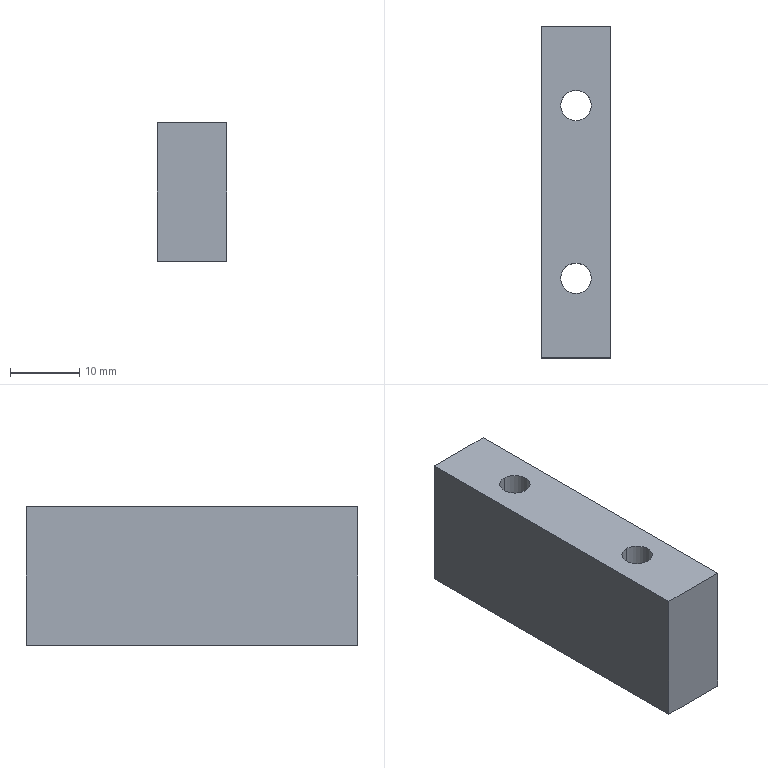Part | SolidWorks | features Extrusion 1, HoleWzd 1 | 1 solid | 16 faces | box 10 x 48 x 20 mm | volume 8641 mm3 | cylinder 8 | plane 8 | commonest cylinder face diameters 4.4 x4 8 x4
STEP:
#1=CARTESIAN_POINT('',(5.,-16.5,-5.));
#2=VERTEX_POINT('',#1);
#3=CARTESIAN_POINT('',(5.,-8.5,-5.));
#4=VERTEX_POINT('',#3);
#5=CARTESIAN_POINT('',(5.,-12.5,-5.));
#6=DIRECTION('',(0.,0.,-1.));
#7=DIRECTION('',(0.,1.,0.));
#8=AXIS2_PLACEMENT_3D('',#5,#6,#7);
#9=CIRCLE('',#8,4.);
#10=EDGE_CURVE('',#2,#4,#9,.T.);
#11=ORIENTED_EDGE('',*,*,#10,.F.);
#12=CARTESIAN_POINT('',(5.,-16.5,-10.));
#13=VERTEX_POINT('',#12);
#14=CARTESIAN_POINT('',(5.,-16.5,-10.));
#15=DIRECTION('',(0.,0.,-1.));
#16=VECTOR('',#15,1000.);
#17=LINE('',#14,#16);
#18=EDGE_CURVE('',#2,#13,#17,.T.);
#19=ORIENTED_EDGE('',*,*,#18,.T.);
#20=CARTESIAN_POINT('',(5.,-8.5,-10.));
#21=VERTEX_POINT('',#20);
#22=CARTESIAN_POINT('',(5.,-12.5,-10.));
#23=DIRECTION('',(0.,0.,-1.));
#24=DIRECTION('',(0.,1.,0.));
#25=AXIS2_PLACEMENT_3D('',#22,#23,#24);
#26=CIRCLE('',#25,4.);
#27=EDGE_CURVE('',#13,#21,#26,.T.);
#28=ORIENTED_EDGE('',*,*,#27,.T.);
#29=CARTESIAN_POINT('',(5.,-8.5,-10.));
#30=DIRECTION('',(0.,0.,-1.));
#31=VECTOR('',#30,1000.);
#32=LINE('',#29,#31);
#33=EDGE_CURVE('',#4,#21,#32,.T.);
#34=ORIENTED_EDGE('',*,*,#33,.F.);
#35=EDGE_LOOP('',(#11,#19,#28,#34));
#36=FACE_OUTER_BOUND('',#35,.T.);
#37=CARTESIAN_POINT('',(5.,-12.5,-10.));
#38=DIRECTION('',(0.,0.,-1.));
#39=DIRECTION('',(0.,1.,0.));
#40=AXIS2_PLACEMENT_3D('',#37,#38,#39);
#41=CYLINDRICAL_SURFACE('',#40,4.);
#42=ADVANCED_FACE('',(#36),#41,.F.);
#43=CARTESIAN_POINT('',(5.,-14.7,10.));
#44=VERTEX_POINT('',#43);
#45=CARTESIAN_POINT('',(5.,-10.3,10.));
#46=VERTEX_POINT('',#45);
#47=CARTESIAN_POINT('',(5.,-12.5,10.));
#48=DIRECTION('',(0.,0.,-1.));
#49=DIRECTION('',(0.,1.,0.));
#50=AXIS2_PLACEMENT_3D('',#47,#48,#49);
#51=CIRCLE('',#50,2.2);
#52=EDGE_CURVE('',#44,#46,#51,.T.);
#53=ORIENTED_EDGE('',*,*,#52,.F.);
#54=CARTESIAN_POINT('',(5.,-14.7,-5.));
#55=VERTEX_POINT('',#54);
#56=CARTESIAN_POINT('',(5.,-14.7,-10.));
#57=DIRECTION('',(0.,0.,-1.));
#58=VECTOR('',#57,1000.);
#59=LINE('',#56,#58);
#60=EDGE_CURVE('',#44,#55,#59,.T.);
#61=ORIENTED_EDGE('',*,*,#60,.T.);
#62=CARTESIAN_POINT('',(5.,-10.3,-5.));
#63=VERTEX_POINT('',#62);
#64=CARTESIAN_POINT('',(5.,-12.5,-5.));
#65=DIRECTION('',(0.,0.,-1.));
#66=DIRECTION('',(0.,1.,0.));
#67=AXIS2_PLACEMENT_3D('',#64,#65,#66);
#68=CIRCLE('',#67,2.2);
#69=EDGE_CURVE('',#55,#63,#68,.T.);
#70=ORIENTED_EDGE('',*,*,#69,.T.);
#71=CARTESIAN_POINT('',(5.,-10.3,-10.));
#72=DIRECTION('',(0.,0.,-1.));
#73=VECTOR('',#72,1000.);
#74=LINE('',#71,#73);
#75=EDGE_CURVE('',#46,#63,#74,.T.);
#76=ORIENTED_EDGE('',*,*,#75,.F.);
#77=EDGE_LOOP('',(#53,#61,#70,#76));
#78=FACE_OUTER_BOUND('',#77,.T.);
#79=CARTESIAN_POINT('',(5.,-12.5,-10.));
#80=DIRECTION('',(0.,0.,-1.));
#81=DIRECTION('',(0.,1.,0.));
#82=AXIS2_PLACEMENT_3D('',#79,#80,#81);
#83=CYLINDRICAL_SURFACE('',#82,2.2);
#84=ADVANCED_FACE('',(#78),#83,.F.);
#85=CARTESIAN_POINT('',(5.,8.5,-5.));
#86=VERTEX_POINT('',#85);
#87=CARTESIAN_POINT('',(5.,16.5,-5.));
#88=VERTEX_POINT('',#87);
#89=CARTESIAN_POINT('',(5.,12.5,-5.));
#90=DIRECTION('',(0.,0.,-1.));
#91=DIRECTION('',(0.,1.,0.));
#92=AXIS2_PLACEMENT_3D('',#89,#90,#91);
#93=CIRCLE('',#92,4.);
#94=EDGE_CURVE('',#86,#88,#93,.T.);
#95=ORIENTED_EDGE('',*,*,#94,.F.);
#96=CARTESIAN_POINT('',(5.,8.5,-10.));
#97=VERTEX_POINT('',#96);
#98=CARTESIAN_POINT('',(5.,8.5,-10.));
#99=DIRECTION('',(0.,0.,-1.));
#100=VECTOR('',#99,1000.);
#101=LINE('',#98,#100);
#102=EDGE_CURVE('',#86,#97,#101,.T.);
#103=ORIENTED_EDGE('',*,*,#102,.T.);
#104=CARTESIAN_POINT('',(5.,16.5,-10.));
#105=VERTEX_POINT('',#104);
#106=CARTESIAN_POINT('',(5.,12.5,-10.));
#107=DIRECTION('',(0.,0.,-1.));
#108=DIRECTION('',(0.,1.,0.));
#109=AXIS2_PLACEMENT_3D('',#106,#107,#108);
#110=CIRCLE('',#109,4.);
#111=EDGE_CURVE('',#97,#105,#110,.T.);
#112=ORIENTED_EDGE('',*,*,#111,.T.);
#113=CARTESIAN_POINT('',(5.,16.5,-10.));
#114=DIRECTION('',(0.,0.,-1.));
#115=VECTOR('',#114,1000.);
#116=LINE('',#113,#115);
#117=EDGE_CURVE('',#88,#105,#116,.T.);
#118=ORIENTED_EDGE('',*,*,#117,.F.);
#119=EDGE_LOOP('',(#95,#103,#112,#118));
#120=FACE_OUTER_BOUND('',#119,.T.);
#121=CARTESIAN_POINT('',(5.,12.5,-10.));
#122=DIRECTION('',(0.,0.,-1.));
#123=DIRECTION('',(0.,1.,0.));
#124=AXIS2_PLACEMENT_3D('',#121,#122,#123);
#125=CYLINDRICAL_SURFACE('',#124,4.);
#126=ADVANCED_FACE('',(#120),#125,.F.);
#127=CARTESIAN_POINT('',(5.,10.3,10.));
#128=VERTEX_POINT('',#127);
#129=CARTESIAN_POINT('',(5.,14.7,10.));
#130=VERTEX_POINT('',#129);
#131=CARTESIAN_POINT('',(5.,12.5,10.));
#132=DIRECTION('',(0.,0.,-1.));
#133=DIRECTION('',(0.,1.,0.));
#134=AXIS2_PLACEMENT_3D('',#131,#132,#133);
#135=CIRCLE('',#134,2.2);
#136=EDGE_CURVE('',#128,#130,#135,.T.);
#137=ORIENTED_EDGE('',*,*,#136,.F.);
#138=CARTESIAN_POINT('',(5.,10.3,-5.));
#139=VERTEX_POINT('',#138);
#140=CARTESIAN_POINT('',(5.,10.3,-10.));
#141=DIRECTION('',(0.,0.,-1.));
#142=VECTOR('',#141,1000.);
#143=LINE('',#140,#142);
#144=EDGE_CURVE('',#128,#139,#143,.T.);
#145=ORIENTED_EDGE('',*,*,#144,.T.);
#146=CARTESIAN_POINT('',(5.,14.7,-5.));
#147=VERTEX_POINT('',#146);
#148=CARTESIAN_POINT('',(5.,12.5,-5.));
#149=DIRECTION('',(0.,0.,-1.));
#150=DIRECTION('',(0.,1.,0.));
#151=AXIS2_PLACEMENT_3D('',#148,#149,#150);
#152=CIRCLE('',#151,2.2);
#153=EDGE_CURVE('',#139,#147,#152,.T.);
#154=ORIENTED_EDGE('',*,*,#153,.T.);
#155=CARTESIAN_POINT('',(5.,14.7,-10.));
#156=DIRECTION('',(0.,0.,-1.));
#157=VECTOR('',#156,1000.);
#158=LINE('',#155,#157);
#159=EDGE_CURVE('',#130,#147,#158,.T.);
#160=ORIENTED_EDGE('',*,*,#159,.F.);
#161=EDGE_LOOP('',(#137,#145,#154,#160));
#162=FACE_OUTER_BOUND('',#161,.T.);
#163=CARTESIAN_POINT('',(5.,12.5,-10.));
#164=DIRECTION('',(0.,0.,-1.));
#165=DIRECTION('',(0.,1.,0.));
#166=AXIS2_PLACEMENT_3D('',#163,#164,#165);
#167=CYLINDRICAL_SURFACE('',#166,2.2);
#168=ADVANCED_FACE('',(#162),#167,.F.);
#169=CARTESIAN_POINT('',(5.,-12.5,-10.));
#170=DIRECTION('',(0.,0.,-1.));
#171=DIRECTION('',(0.,1.,0.));
#172=AXIS2_PLACEMENT_3D('',#169,#170,#171);
#173=CIRCLE('',#172,4.);
#174=EDGE_CURVE('',#21,#13,#173,.T.);
#175=ORIENTED_EDGE('',*,*,#174,.F.);
#176=ORIENTED_EDGE('',*,*,#27,.F.);
#177=EDGE_LOOP('',(#175,#176));
#178=FACE_BOUND('',#177,.T.);
#179=CARTESIAN_POINT('',(5.,12.5,-10.));
#180=DIRECTION('',(0.,0.,-1.));
#181=DIRECTION('',(0.,1.,0.));
#182=AXIS2_PLACEMENT_3D('',#179,#180,#181);
#183=CIRCLE('',#182,4.);
#184=EDGE_CURVE('',#105,#97,#183,.T.);
#185=ORIENTED_EDGE('',*,*,#184,.F.);
#186=ORIENTED_EDGE('',*,*,#111,.F.);
#187=EDGE_LOOP('',(#185,#186));
#188=FACE_BOUND('',#187,.T.);
#189=CARTESIAN_POINT('',(0.,-24.,-10.));
#190=VERTEX_POINT('',#189);
#191=CARTESIAN_POINT('',(0.,24.,-10.));
#192=VERTEX_POINT('',#191);
#193=CARTESIAN_POINT('',(0.,24.,-10.));
#194=DIRECTION('',(0.,1.,0.));
#195=VECTOR('',#194,1000.);
#196=LINE('',#193,#195);
#197=EDGE_CURVE('',#190,#192,#196,.T.);
#198=ORIENTED_EDGE('',*,*,#197,.T.);
#199=CARTESIAN_POINT('',(10.,24.,-10.));
#200=VERTEX_POINT('',#199);
#201=CARTESIAN_POINT('',(10.,24.,-10.));
#202=DIRECTION('',(-1.,0.,0.));
#203=VECTOR('',#202,1000.);
#204=LINE('',#201,#203);
#205=EDGE_CURVE('',#200,#192,#204,.T.);
#206=ORIENTED_EDGE('',*,*,#205,.F.);
#207=CARTESIAN_POINT('',(10.,-24.,-10.));
#208=VERTEX_POINT('',#207);
#209=CARTESIAN_POINT('',(10.,24.,-10.));
#210=DIRECTION('',(0.,1.,0.));
#211=VECTOR('',#210,1000.);
#212=LINE('',#209,#211);
#213=EDGE_CURVE('',#208,#200,#212,.T.);
#214=ORIENTED_EDGE('',*,*,#213,.F.);
#215=CARTESIAN_POINT('',(10.,-24.,-10.));
#216=DIRECTION('',(-1.,0.,0.));
#217=VECTOR('',#216,1000.);
#218=LINE('',#215,#217);
#219=EDGE_CURVE('',#208,#190,#218,.T.);
#220=ORIENTED_EDGE('',*,*,#219,.T.);
#221=EDGE_LOOP('',(#198,#206,#214,#220));
#222=FACE_OUTER_BOUND('',#221,.T.);
#223=CARTESIAN_POINT('',(10.,24.,-10.));
#224=DIRECTION('',(0.,0.,1.));
#225=DIRECTION('',(0.,-1.,0.));
#226=AXIS2_PLACEMENT_3D('',#223,#224,#225);
#227=PLANE('',#226);
#228=ADVANCED_FACE('',(#178,#188,#222),#227,.F.);
#229=CARTESIAN_POINT('',(0.,24.,10.));
#230=VERTEX_POINT('',#229);
#231=CARTESIAN_POINT('',(0.,24.,10.));
#232=DIRECTION('',(0.,0.,1.));
#233=VECTOR('',#232,1000.);
#234=LINE('',#231,#233);
#235=EDGE_CURVE('',#192,#230,#234,.T.);
#236=ORIENTED_EDGE('',*,*,#235,.T.);
#237=CARTESIAN_POINT('',(10.,24.,10.));
#238=VERTEX_POINT('',#237);
#239=CARTESIAN_POINT('',(10.,24.,10.));
#240=DIRECTION('',(-1.,0.,0.));
#241=VECTOR('',#240,1000.);
#242=LINE('',#239,#241);
#243=EDGE_CURVE('',#238,#230,#242,.T.);
#244=ORIENTED_EDGE('',*,*,#243,.F.);
#245=CARTESIAN_POINT('',(10.,24.,10.));
#246=DIRECTION('',(0.,0.,1.));
#247=VECTOR('',#246,1000.);
#248=LINE('',#245,#247);
#249=EDGE_CURVE('',#200,#238,#248,.T.);
#250=ORIENTED_EDGE('',*,*,#249,.F.);
#251=ORIENTED_EDGE('',*,*,#205,.T.);
#252=EDGE_LOOP('',(#236,#244,#250,#251));
#253=FACE_OUTER_BOUND('',#252,.T.);
#254=CARTESIAN_POINT('',(10.,24.,10.));
#255=DIRECTION('',(0.,-1.,0.));
#256=DIRECTION('',(0.,0.,-1.));
#257=AXIS2_PLACEMENT_3D('',#254,#255,#256);
#258=PLANE('',#257);
#259=ADVANCED_FACE('',(#253),#258,.F.);
#260=CARTESIAN_POINT('',(5.,-12.5,10.));
#261=DIRECTION('',(0.,0.,-1.));
#262=DIRECTION('',(0.,1.,0.));
#263=AXIS2_PLACEMENT_3D('',#260,#261,#262);
#264=CIRCLE('',#263,2.2);
#265=EDGE_CURVE('',#46,#44,#264,.T.);
#266=ORIENTED_EDGE('',*,*,#265,.T.);
#267=ORIENTED_EDGE('',*,*,#52,.T.);
#268=EDGE_LOOP('',(#266,#267));
#269=FACE_BOUND('',#268,.T.);
#270=CARTESIAN_POINT('',(5.,12.5,10.));
#271=DIRECTION('',(0.,0.,-1.));
#272=DIRECTION('',(0.,1.,0.));
#273=AXIS2_PLACEMENT_3D('',#270,#271,#272);
#274=CIRCLE('',#273,2.2);
#275=EDGE_CURVE('',#130,#128,#274,.T.);
#276=ORIENTED_EDGE('',*,*,#275,.T.);
#277=ORIENTED_EDGE('',*,*,#136,.T.);
#278=EDGE_LOOP('',(#276,#277));
#279=FACE_BOUND('',#278,.T.);
#280=CARTESIAN_POINT('',(0.,-24.,10.));
#281=VERTEX_POINT('',#280);
#282=CARTESIAN_POINT('',(0.,24.,10.));
#283=DIRECTION('',(0.,-1.,0.));
#284=VECTOR('',#283,1000.);
#285=LINE('',#282,#284);
#286=EDGE_CURVE('',#230,#281,#285,.T.);
#287=ORIENTED_EDGE('',*,*,#286,.T.);
#288=CARTESIAN_POINT('',(10.,-24.,10.));
#289=VERTEX_POINT('',#288);
#290=CARTESIAN_POINT('',(10.,-24.,10.));
#291=DIRECTION('',(-1.,0.,0.));
#292=VECTOR('',#291,1000.);
#293=LINE('',#290,#292);
#294=EDGE_CURVE('',#289,#281,#293,.T.);
#295=ORIENTED_EDGE('',*,*,#294,.F.);
#296=CARTESIAN_POINT('',(10.,24.,10.));
#297=DIRECTION('',(0.,-1.,0.));
#298=VECTOR('',#297,1000.);
#299=LINE('',#296,#298);
#300=EDGE_CURVE('',#238,#289,#299,.T.);
#301=ORIENTED_EDGE('',*,*,#300,.F.);
#302=ORIENTED_EDGE('',*,*,#243,.T.);
#303=EDGE_LOOP('',(#287,#295,#301,#302));
#304=FACE_OUTER_BOUND('',#303,.T.);
#305=CARTESIAN_POINT('',(10.,24.,10.));
#306=DIRECTION('',(0.,0.,-1.));
#307=DIRECTION('',(0.,1.,0.));
#308=AXIS2_PLACEMENT_3D('',#305,#306,#307);
#309=PLANE('',#308);
#310=ADVANCED_FACE('',(#269,#279,#304),#309,.F.);
#311=CARTESIAN_POINT('',(0.,-24.,10.));
#312=DIRECTION('',(0.,0.,-1.));
#313=VECTOR('',#312,1000.);
#314=LINE('',#311,#313);
#315=EDGE_CURVE('',#281,#190,#314,.T.);
#316=ORIENTED_EDGE('',*,*,#315,.T.);
#317=ORIENTED_EDGE('',*,*,#219,.F.);
#318=CARTESIAN_POINT('',(10.,-24.,10.));
#319=DIRECTION('',(0.,0.,-1.));
#320=VECTOR('',#319,1000.);
#321=LINE('',#318,#320);
#322=EDGE_CURVE('',#289,#208,#321,.T.);
#323=ORIENTED_EDGE('',*,*,#322,.F.);
#324=ORIENTED_EDGE('',*,*,#294,.T.);
#325=EDGE_LOOP('',(#316,#317,#323,#324));
#326=FACE_OUTER_BOUND('',#325,.T.);
#327=CARTESIAN_POINT('',(10.,-24.,10.));
#328=DIRECTION('',(0.,1.,0.));
#329=DIRECTION('',(0.,0.,1.));
#330=AXIS2_PLACEMENT_3D('',#327,#328,#329);
#331=PLANE('',#330);
#332=ADVANCED_FACE('',(#326),#331,.F.);
#333=ORIENTED_EDGE('',*,*,#213,.T.);
#334=ORIENTED_EDGE('',*,*,#249,.T.);
#335=ORIENTED_EDGE('',*,*,#300,.T.);
#336=ORIENTED_EDGE('',*,*,#322,.T.);
#337=EDGE_LOOP('',(#333,#334,#335,#336));
#338=FACE_OUTER_BOUND('',#337,.T.);
#339=CARTESIAN_POINT('',(10.,0.,0.));
#340=DIRECTION('',(1.,0.,0.));
#341=DIRECTION('',(0.,0.,-1.));
#342=AXIS2_PLACEMENT_3D('',#339,#340,#341);
#343=PLANE('',#342);
#344=ADVANCED_FACE('',(#338),#343,.T.);
#345=ORIENTED_EDGE('',*,*,#197,.F.);
#346=ORIENTED_EDGE('',*,*,#315,.F.);
#347=ORIENTED_EDGE('',*,*,#286,.F.);
#348=ORIENTED_EDGE('',*,*,#235,.F.);
#349=EDGE_LOOP('',(#345,#346,#347,#348));
#350=FACE_OUTER_BOUND('',#349,.T.);
#351=CARTESIAN_POINT('',(0.,0.,0.));
#352=DIRECTION('',(1.,0.,0.));
#353=DIRECTION('',(0.,0.,-1.));
#354=AXIS2_PLACEMENT_3D('',#351,#352,#353);
#355=PLANE('',#354);
#356=ADVANCED_FACE('',(#350),#355,.F.);
#357=ORIENTED_EDGE('',*,*,#144,.F.);
#358=ORIENTED_EDGE('',*,*,#275,.F.);
#359=ORIENTED_EDGE('',*,*,#159,.T.);
#360=CARTESIAN_POINT('',(5.,12.5,-5.));
#361=DIRECTION('',(0.,0.,-1.));
#362=DIRECTION('',(0.,1.,0.));
#363=AXIS2_PLACEMENT_3D('',#360,#361,#362);
#364=CIRCLE('',#363,2.2);
#365=EDGE_CURVE('',#147,#139,#364,.T.);
#366=ORIENTED_EDGE('',*,*,#365,.T.);
#367=EDGE_LOOP('',(#357,#358,#359,#366));
#368=FACE_OUTER_BOUND('',#367,.T.);
#369=CARTESIAN_POINT('',(5.,12.5,-10.));
#370=DIRECTION('',(0.,0.,-1.));
#371=DIRECTION('',(0.,1.,0.));
#372=AXIS2_PLACEMENT_3D('',#369,#370,#371);
#373=CYLINDRICAL_SURFACE('',#372,2.2);
#374=ADVANCED_FACE('',(#368),#373,.F.);
#375=ORIENTED_EDGE('',*,*,#365,.F.);
#376=ORIENTED_EDGE('',*,*,#153,.F.);
#377=EDGE_LOOP('',(#375,#376));
#378=FACE_BOUND('',#377,.T.);
#379=CARTESIAN_POINT('',(5.,12.5,-5.));
#380=DIRECTION('',(0.,0.,-1.));
#381=DIRECTION('',(0.,1.,0.));
#382=AXIS2_PLACEMENT_3D('',#379,#380,#381);
#383=CIRCLE('',#382,4.);
#384=EDGE_CURVE('',#88,#86,#383,.T.);
#385=ORIENTED_EDGE('',*,*,#384,.T.);
#386=ORIENTED_EDGE('',*,*,#94,.T.);
#387=EDGE_LOOP('',(#385,#386));
#388=FACE_OUTER_BOUND('',#387,.T.);
#389=CARTESIAN_POINT('',(7.2,12.5,-5.));
#390=DIRECTION('',(0.,0.,1.));
#391=DIRECTION('',(0.,-1.,0.));
#392=AXIS2_PLACEMENT_3D('',#389,#390,#391);
#393=PLANE('',#392);
#394=ADVANCED_FACE('',(#378,#388),#393,.F.);
#395=ORIENTED_EDGE('',*,*,#102,.F.);
#396=ORIENTED_EDGE('',*,*,#384,.F.);
#397=ORIENTED_EDGE('',*,*,#117,.T.);
#398=ORIENTED_EDGE('',*,*,#184,.T.);
#399=EDGE_LOOP('',(#395,#396,#397,#398));
#400=FACE_OUTER_BOUND('',#399,.T.);
#401=CARTESIAN_POINT('',(5.,12.5,-10.));
#402=DIRECTION('',(0.,0.,-1.));
#403=DIRECTION('',(0.,1.,0.));
#404=AXIS2_PLACEMENT_3D('',#401,#402,#403);
#405=CYLINDRICAL_SURFACE('',#404,4.);
#406=ADVANCED_FACE('',(#400),#405,.F.);
#407=ORIENTED_EDGE('',*,*,#60,.F.);
#408=ORIENTED_EDGE('',*,*,#265,.F.);
#409=ORIENTED_EDGE('',*,*,#75,.T.);
#410=CARTESIAN_POINT('',(5.,-12.5,-5.));
#411=DIRECTION('',(0.,0.,-1.));
#412=DIRECTION('',(0.,1.,0.));
#413=AXIS2_PLACEMENT_3D('',#410,#411,#412);
#414=CIRCLE('',#413,2.2);
#415=EDGE_CURVE('',#63,#55,#414,.T.);
#416=ORIENTED_EDGE('',*,*,#415,.T.);
#417=EDGE_LOOP('',(#407,#408,#409,#416));
#418=FACE_OUTER_BOUND('',#417,.T.);
#419=CARTESIAN_POINT('',(5.,-12.5,-10.));
#420=DIRECTION('',(0.,0.,-1.));
#421=DIRECTION('',(0.,1.,0.));
#422=AXIS2_PLACEMENT_3D('',#419,#420,#421);
#423=CYLINDRICAL_SURFACE('',#422,2.2);
#424=ADVANCED_FACE('',(#418),#423,.F.);
#425=ORIENTED_EDGE('',*,*,#415,.F.);
#426=ORIENTED_EDGE('',*,*,#69,.F.);
#427=EDGE_LOOP('',(#425,#426));
#428=FACE_BOUND('',#427,.T.);
#429=CARTESIAN_POINT('',(5.,-12.5,-5.));
#430=DIRECTION('',(0.,0.,-1.));
#431=DIRECTION('',(0.,1.,0.));
#432=AXIS2_PLACEMENT_3D('',#429,#430,#431);
#433=CIRCLE('',#432,4.);
#434=EDGE_CURVE('',#4,#2,#433,.T.);
#435=ORIENTED_EDGE('',*,*,#434,.T.);
#436=ORIENTED_EDGE('',*,*,#10,.T.);
#437=EDGE_LOOP('',(#435,#436));
#438=FACE_OUTER_BOUND('',#437,.T.);
#439=CARTESIAN_POINT('',(7.2,-12.5,-5.));
#440=DIRECTION('',(0.,0.,1.));
#441=DIRECTION('',(0.,-1.,0.));
#442=AXIS2_PLACEMENT_3D('',#439,#440,#441);
#443=PLANE('',#442);
#444=ADVANCED_FACE('',(#428,#438),#443,.F.);
#445=ORIENTED_EDGE('',*,*,#18,.F.);
#446=ORIENTED_EDGE('',*,*,#434,.F.);
#447=ORIENTED_EDGE('',*,*,#33,.T.);
#448=ORIENTED_EDGE('',*,*,#174,.T.);
#449=EDGE_LOOP('',(#445,#446,#447,#448));
#450=FACE_OUTER_BOUND('',#449,.T.);
#451=CARTESIAN_POINT('',(5.,-12.5,-10.));
#452=DIRECTION('',(0.,0.,-1.));
#453=DIRECTION('',(0.,1.,0.));
#454=AXIS2_PLACEMENT_3D('',#451,#452,#453);
#455=CYLINDRICAL_SURFACE('',#454,4.);
#456=ADVANCED_FACE('',(#450),#455,.F.);
#457=CLOSED_SHELL('',(#42,#84,#126,#168,#228,#259,#310,#332,#344,#356,#374,#394,#406,#424,#444,#456));
#458=MANIFOLD_SOLID_BREP('',#457);
#459=CARTESIAN_POINT('',(0.,0.,0.));
#460=DIRECTION('',(0.,0.,1.));
#461=DIRECTION('',(1.,0.,0.));
#462=AXIS2_PLACEMENT_3D('',#459,#460,#461);
#463=(LENGTH_UNIT()NAMED_UNIT(*)SI_UNIT(.MILLI.,.METRE.));
#464=UNCERTAINTY_MEASURE_WITH_UNIT(LENGTH_MEASURE(0.00001),#463,'','');
#465=(NAMED_UNIT(*)PLANE_ANGLE_UNIT()SI_UNIT($,.RADIAN.));
#466=(NAMED_UNIT(*)SI_UNIT($,.STERADIAN.)SOLID_ANGLE_UNIT());
#467=(GEOMETRIC_REPRESENTATION_CONTEXT(3)GLOBAL_UNCERTAINTY_ASSIGNED_CONTEXT((#464))GLOBAL_UNIT_ASSIGNED_CONTEXT((#463,#465,#466))REPRESENTATION_CONTEXT('',''));
#468=ADVANCED_BREP_SHAPE_REPRESENTATION('',(#458,#462),#467);